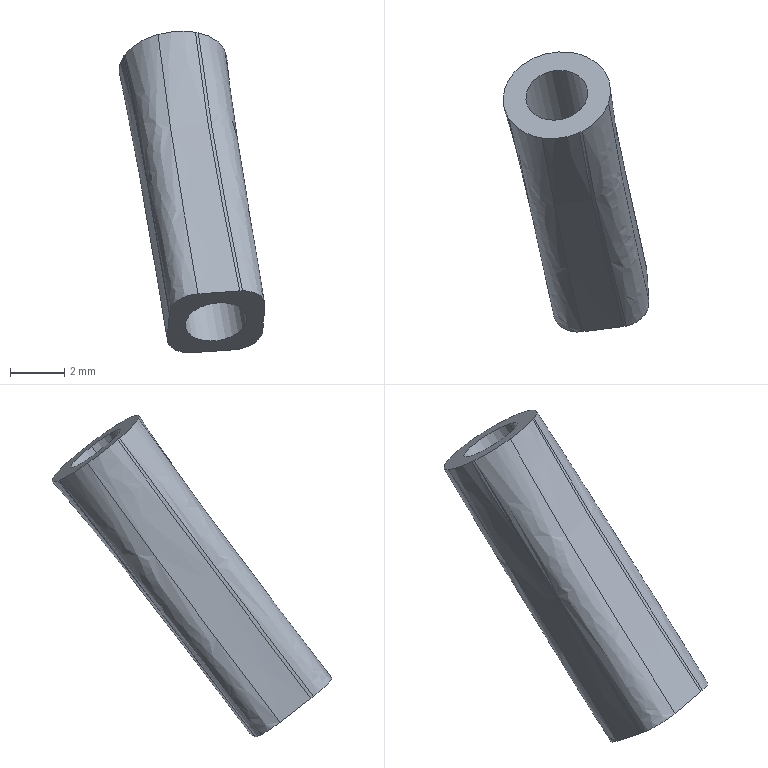Part | STEP file | BREP_16 | 1 solid | 16 faces | box 5.376 x 10.304 x 11.842 mm | volume 92.736 mm3 | spline 12 | plane 2 | cylinder 2 | commonest cylinder face diameters 2.3 x2